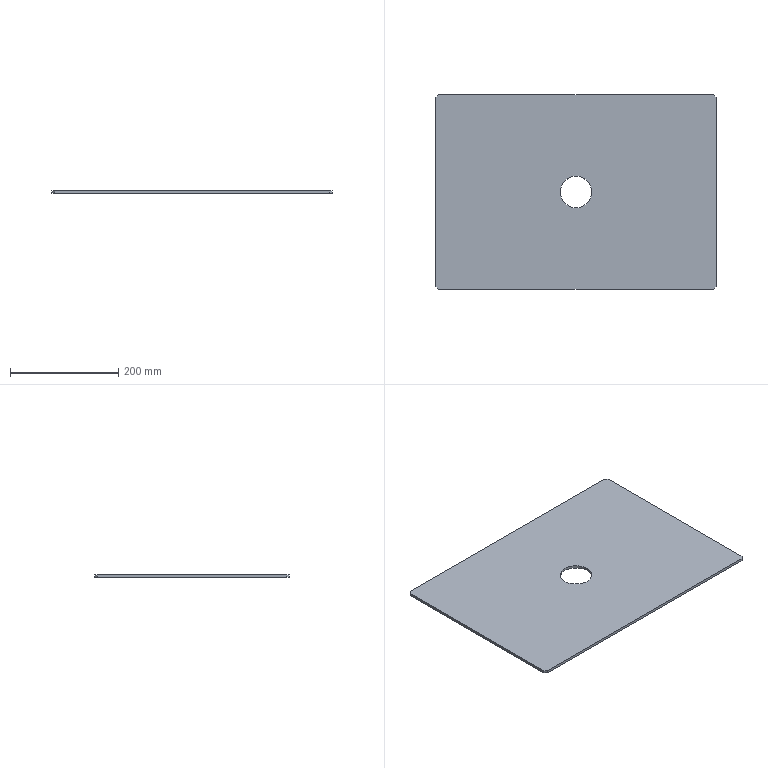Part | SolidWorks | features BaseBody 1 | 1 solid | 12 faces | box 518 x 360 x 5 mm | volume 918757 mm3 | plane 10 | cylinder 2 | commonest cylinder face diameters 58.4 x2
STEP:
#1=CARTESIAN_POINT('',(-29.2,0.,8.5));
#2=VERTEX_POINT('',#1);
#3=CARTESIAN_POINT('',(29.2,0.,8.5));
#4=VERTEX_POINT('',#3);
#5=CARTESIAN_POINT('',(0.,0.,8.5));
#6=DIRECTION('',(0.,0.,1.));
#7=DIRECTION('',(-1.,0.,0.));
#8=AXIS2_PLACEMENT_3D('',#5,#6,#7);
#9=CIRCLE('',#8,29.2);
#10=EDGE_CURVE('',#2,#4,#9,.T.);
#11=ORIENTED_EDGE('',*,*,#10,.T.);
#12=CARTESIAN_POINT('',(29.2,0.,3.5));
#13=VERTEX_POINT('',#12);
#14=CARTESIAN_POINT('',(29.2,0.,8.5));
#15=DIRECTION('',(0.,0.,-1.));
#16=VECTOR('',#15,1000.);
#17=LINE('',#14,#16);
#18=EDGE_CURVE('',#4,#13,#17,.T.);
#19=ORIENTED_EDGE('',*,*,#18,.T.);
#20=CARTESIAN_POINT('',(-29.2,0.,3.5));
#21=VERTEX_POINT('',#20);
#22=CARTESIAN_POINT('',(0.,0.,3.5));
#23=DIRECTION('',(0.,0.,1.));
#24=DIRECTION('',(-1.,0.,0.));
#25=AXIS2_PLACEMENT_3D('',#22,#23,#24);
#26=CIRCLE('',#25,29.2);
#27=EDGE_CURVE('',#21,#13,#26,.T.);
#28=ORIENTED_EDGE('',*,*,#27,.F.);
#29=CARTESIAN_POINT('',(-29.2,0.,8.5));
#30=DIRECTION('',(0.,0.,-1.));
#31=VECTOR('',#30,1000.);
#32=LINE('',#29,#31);
#33=EDGE_CURVE('',#2,#21,#32,.T.);
#34=ORIENTED_EDGE('',*,*,#33,.F.);
#35=EDGE_LOOP('',(#11,#19,#28,#34));
#36=FACE_OUTER_BOUND('',#35,.T.);
#37=CARTESIAN_POINT('',(0.,0.,8.5));
#38=DIRECTION('',(0.,0.,-1.));
#39=DIRECTION('',(-1.,0.,0.));
#40=AXIS2_PLACEMENT_3D('',#37,#38,#39);
#41=CYLINDRICAL_SURFACE('',#40,29.2);
#42=ADVANCED_FACE('',(#36),#41,.F.);
#43=ORIENTED_EDGE('',*,*,#10,.F.);
#44=CARTESIAN_POINT('',(0.,0.,8.5));
#45=DIRECTION('',(0.,0.,1.));
#46=DIRECTION('',(-1.,0.,0.));
#47=AXIS2_PLACEMENT_3D('',#44,#45,#46);
#48=CIRCLE('',#47,29.2);
#49=EDGE_CURVE('',#4,#2,#48,.T.);
#50=ORIENTED_EDGE('',*,*,#49,.F.);
#51=EDGE_LOOP('',(#43,#50));
#52=FACE_BOUND('',#51,.T.);
#53=CARTESIAN_POINT('',(-254.,180.,8.5));
#54=VERTEX_POINT('',#53);
#55=CARTESIAN_POINT('',(254.,180.,8.5));
#56=VERTEX_POINT('',#55);
#57=CARTESIAN_POINT('',(0.,180.,8.5));
#58=DIRECTION('',(1.,0.,0.));
#59=VECTOR('',#58,1000.);
#60=LINE('',#57,#59);
#61=EDGE_CURVE('',#54,#56,#60,.T.);
#62=ORIENTED_EDGE('',*,*,#61,.F.);
#63=CARTESIAN_POINT('',(-259.,175.,8.5));
#64=VERTEX_POINT('',#63);
#65=CARTESIAN_POINT('',(-259.,175.,8.5));
#66=DIRECTION('',(0.7071,0.7071,0.));
#67=VECTOR('',#66,1000.);
#68=LINE('',#65,#67);
#69=EDGE_CURVE('',#64,#54,#68,.T.);
#70=ORIENTED_EDGE('',*,*,#69,.F.);
#71=CARTESIAN_POINT('',(-259.,-175.,8.5));
#72=VERTEX_POINT('',#71);
#73=CARTESIAN_POINT('',(-259.,0.,8.5));
#74=DIRECTION('',(0.,1.,0.));
#75=VECTOR('',#74,1000.);
#76=LINE('',#73,#75);
#77=EDGE_CURVE('',#72,#64,#76,.T.);
#78=ORIENTED_EDGE('',*,*,#77,.F.);
#79=CARTESIAN_POINT('',(-254.,-180.,8.5));
#80=VERTEX_POINT('',#79);
#81=CARTESIAN_POINT('',(-254.,-180.,8.5));
#82=DIRECTION('',(-0.7071,0.7071,0.));
#83=VECTOR('',#82,1000.);
#84=LINE('',#81,#83);
#85=EDGE_CURVE('',#80,#72,#84,.T.);
#86=ORIENTED_EDGE('',*,*,#85,.F.);
#87=CARTESIAN_POINT('',(254.,-180.,8.5));
#88=VERTEX_POINT('',#87);
#89=CARTESIAN_POINT('',(0.,-180.,8.5));
#90=DIRECTION('',(-1.,0.,0.));
#91=VECTOR('',#90,1000.);
#92=LINE('',#89,#91);
#93=EDGE_CURVE('',#88,#80,#92,.T.);
#94=ORIENTED_EDGE('',*,*,#93,.F.);
#95=CARTESIAN_POINT('',(259.,-175.,8.5));
#96=VERTEX_POINT('',#95);
#97=CARTESIAN_POINT('',(259.,-175.,8.5));
#98=DIRECTION('',(-0.7071,-0.7071,0.));
#99=VECTOR('',#98,1000.);
#100=LINE('',#97,#99);
#101=EDGE_CURVE('',#96,#88,#100,.T.);
#102=ORIENTED_EDGE('',*,*,#101,.F.);
#103=CARTESIAN_POINT('',(259.,175.,8.5));
#104=VERTEX_POINT('',#103);
#105=CARTESIAN_POINT('',(259.,0.,8.5));
#106=DIRECTION('',(0.,-1.,0.));
#107=VECTOR('',#106,1000.);
#108=LINE('',#105,#107);
#109=EDGE_CURVE('',#104,#96,#108,.T.);
#110=ORIENTED_EDGE('',*,*,#109,.F.);
#111=CARTESIAN_POINT('',(254.,180.,8.5));
#112=DIRECTION('',(0.7071,-0.7071,0.));
#113=VECTOR('',#112,1000.);
#114=LINE('',#111,#113);
#115=EDGE_CURVE('',#56,#104,#114,.T.);
#116=ORIENTED_EDGE('',*,*,#115,.F.);
#117=EDGE_LOOP('',(#62,#70,#78,#86,#94,#102,#110,#116));
#118=FACE_OUTER_BOUND('',#117,.T.);
#119=CARTESIAN_POINT('',(0.,0.,8.5));
#120=DIRECTION('',(0.,0.,-1.));
#121=DIRECTION('',(-1.,0.,0.));
#122=AXIS2_PLACEMENT_3D('',#119,#120,#121);
#123=PLANE('',#122);
#124=ADVANCED_FACE('',(#52,#118),#123,.F.);
#125=ORIENTED_EDGE('',*,*,#18,.F.);
#126=ORIENTED_EDGE('',*,*,#49,.T.);
#127=ORIENTED_EDGE('',*,*,#33,.T.);
#128=CARTESIAN_POINT('',(0.,0.,3.5));
#129=DIRECTION('',(0.,0.,1.));
#130=DIRECTION('',(-1.,0.,0.));
#131=AXIS2_PLACEMENT_3D('',#128,#129,#130);
#132=CIRCLE('',#131,29.2);
#133=EDGE_CURVE('',#13,#21,#132,.T.);
#134=ORIENTED_EDGE('',*,*,#133,.F.);
#135=EDGE_LOOP('',(#125,#126,#127,#134));
#136=FACE_OUTER_BOUND('',#135,.T.);
#137=CARTESIAN_POINT('',(0.,0.,8.5));
#138=DIRECTION('',(0.,0.,-1.));
#139=DIRECTION('',(-1.,0.,0.));
#140=AXIS2_PLACEMENT_3D('',#137,#138,#139);
#141=CYLINDRICAL_SURFACE('',#140,29.2);
#142=ADVANCED_FACE('',(#136),#141,.F.);
#143=CARTESIAN_POINT('',(259.,175.,3.5));
#144=VERTEX_POINT('',#143);
#145=CARTESIAN_POINT('',(254.,180.,3.5));
#146=VERTEX_POINT('',#145);
#147=CARTESIAN_POINT('',(254.,180.,3.5));
#148=DIRECTION('',(-0.7071,0.7071,0.));
#149=VECTOR('',#148,1000.);
#150=LINE('',#147,#149);
#151=EDGE_CURVE('',#144,#146,#150,.T.);
#152=ORIENTED_EDGE('',*,*,#151,.T.);
#153=CARTESIAN_POINT('',(254.,180.,8.5));
#154=DIRECTION('',(0.,0.,1.));
#155=VECTOR('',#154,1000.);
#156=LINE('',#153,#155);
#157=EDGE_CURVE('',#146,#56,#156,.T.);
#158=ORIENTED_EDGE('',*,*,#157,.T.);
#159=ORIENTED_EDGE('',*,*,#115,.T.);
#160=CARTESIAN_POINT('',(259.,175.,8.5));
#161=DIRECTION('',(0.,0.,-1.));
#162=VECTOR('',#161,1000.);
#163=LINE('',#160,#162);
#164=EDGE_CURVE('',#104,#144,#163,.T.);
#165=ORIENTED_EDGE('',*,*,#164,.T.);
#166=EDGE_LOOP('',(#152,#158,#159,#165));
#167=FACE_OUTER_BOUND('',#166,.T.);
#168=CARTESIAN_POINT('',(254.,180.,8.5));
#169=DIRECTION('',(0.7071,0.7071,0.));
#170=DIRECTION('',(-0.7071,0.7071,0.));
#171=AXIS2_PLACEMENT_3D('',#168,#169,#170);
#172=PLANE('',#171);
#173=ADVANCED_FACE('',(#167),#172,.T.);
#174=CARTESIAN_POINT('',(-254.,180.,3.5));
#175=VERTEX_POINT('',#174);
#176=CARTESIAN_POINT('',(-254.,180.,3.5));
#177=DIRECTION('',(-1.,0.,0.));
#178=VECTOR('',#177,1000.);
#179=LINE('',#176,#178);
#180=EDGE_CURVE('',#146,#175,#179,.T.);
#181=ORIENTED_EDGE('',*,*,#180,.T.);
#182=CARTESIAN_POINT('',(-254.,180.,8.5));
#183=DIRECTION('',(0.,0.,1.));
#184=VECTOR('',#183,1000.);
#185=LINE('',#182,#184);
#186=EDGE_CURVE('',#175,#54,#185,.T.);
#187=ORIENTED_EDGE('',*,*,#186,.T.);
#188=ORIENTED_EDGE('',*,*,#61,.T.);
#189=ORIENTED_EDGE('',*,*,#157,.F.);
#190=EDGE_LOOP('',(#181,#187,#188,#189));
#191=FACE_OUTER_BOUND('',#190,.T.);
#192=CARTESIAN_POINT('',(-254.,180.,8.5));
#193=DIRECTION('',(0.,1.,0.));
#194=DIRECTION('',(0.,0.,1.));
#195=AXIS2_PLACEMENT_3D('',#192,#193,#194);
#196=PLANE('',#195);
#197=ADVANCED_FACE('',(#191),#196,.T.);
#198=CARTESIAN_POINT('',(-259.,175.,3.5));
#199=VERTEX_POINT('',#198);
#200=CARTESIAN_POINT('',(-259.,175.,3.5));
#201=DIRECTION('',(-0.7071,-0.7071,0.));
#202=VECTOR('',#201,1000.);
#203=LINE('',#200,#202);
#204=EDGE_CURVE('',#175,#199,#203,.T.);
#205=ORIENTED_EDGE('',*,*,#204,.T.);
#206=CARTESIAN_POINT('',(-259.,175.,8.5));
#207=DIRECTION('',(0.,0.,1.));
#208=VECTOR('',#207,1000.);
#209=LINE('',#206,#208);
#210=EDGE_CURVE('',#199,#64,#209,.T.);
#211=ORIENTED_EDGE('',*,*,#210,.T.);
#212=ORIENTED_EDGE('',*,*,#69,.T.);
#213=ORIENTED_EDGE('',*,*,#186,.F.);
#214=EDGE_LOOP('',(#205,#211,#212,#213));
#215=FACE_OUTER_BOUND('',#214,.T.);
#216=CARTESIAN_POINT('',(-259.,175.,8.5));
#217=DIRECTION('',(-0.7071,0.7071,0.));
#218=DIRECTION('',(-0.7071,-0.7071,0.));
#219=AXIS2_PLACEMENT_3D('',#216,#217,#218);
#220=PLANE('',#219);
#221=ADVANCED_FACE('',(#215),#220,.T.);
#222=CARTESIAN_POINT('',(-259.,-175.,3.5));
#223=VERTEX_POINT('',#222);
#224=CARTESIAN_POINT('',(-259.,-175.,3.5));
#225=DIRECTION('',(0.,-1.,0.));
#226=VECTOR('',#225,1000.);
#227=LINE('',#224,#226);
#228=EDGE_CURVE('',#199,#223,#227,.T.);
#229=ORIENTED_EDGE('',*,*,#228,.T.);
#230=CARTESIAN_POINT('',(-259.,-175.,8.5));
#231=DIRECTION('',(0.,0.,1.));
#232=VECTOR('',#231,1000.);
#233=LINE('',#230,#232);
#234=EDGE_CURVE('',#223,#72,#233,.T.);
#235=ORIENTED_EDGE('',*,*,#234,.T.);
#236=ORIENTED_EDGE('',*,*,#77,.T.);
#237=ORIENTED_EDGE('',*,*,#210,.F.);
#238=EDGE_LOOP('',(#229,#235,#236,#237));
#239=FACE_OUTER_BOUND('',#238,.T.);
#240=CARTESIAN_POINT('',(-259.,-175.,8.5));
#241=DIRECTION('',(-1.,0.,0.));
#242=DIRECTION('',(0.,0.,1.));
#243=AXIS2_PLACEMENT_3D('',#240,#241,#242);
#244=PLANE('',#243);
#245=ADVANCED_FACE('',(#239),#244,.T.);
#246=CARTESIAN_POINT('',(-254.,-180.,3.5));
#247=VERTEX_POINT('',#246);
#248=CARTESIAN_POINT('',(-254.,-180.,3.5));
#249=DIRECTION('',(0.7071,-0.7071,0.));
#250=VECTOR('',#249,1000.);
#251=LINE('',#248,#250);
#252=EDGE_CURVE('',#223,#247,#251,.T.);
#253=ORIENTED_EDGE('',*,*,#252,.T.);
#254=CARTESIAN_POINT('',(-254.,-180.,8.5));
#255=DIRECTION('',(0.,0.,1.));
#256=VECTOR('',#255,1000.);
#257=LINE('',#254,#256);
#258=EDGE_CURVE('',#247,#80,#257,.T.);
#259=ORIENTED_EDGE('',*,*,#258,.T.);
#260=ORIENTED_EDGE('',*,*,#85,.T.);
#261=ORIENTED_EDGE('',*,*,#234,.F.);
#262=EDGE_LOOP('',(#253,#259,#260,#261));
#263=FACE_OUTER_BOUND('',#262,.T.);
#264=CARTESIAN_POINT('',(-254.,-180.,8.5));
#265=DIRECTION('',(-0.7071,-0.7071,0.));
#266=DIRECTION('',(0.7071,-0.7071,0.));
#267=AXIS2_PLACEMENT_3D('',#264,#265,#266);
#268=PLANE('',#267);
#269=ADVANCED_FACE('',(#263),#268,.T.);
#270=CARTESIAN_POINT('',(254.,-180.,3.5));
#271=VERTEX_POINT('',#270);
#272=CARTESIAN_POINT('',(254.,-180.,3.5));
#273=DIRECTION('',(1.,0.,0.));
#274=VECTOR('',#273,1000.);
#275=LINE('',#272,#274);
#276=EDGE_CURVE('',#247,#271,#275,.T.);
#277=ORIENTED_EDGE('',*,*,#276,.T.);
#278=CARTESIAN_POINT('',(254.,-180.,8.5));
#279=DIRECTION('',(0.,0.,1.));
#280=VECTOR('',#279,1000.);
#281=LINE('',#278,#280);
#282=EDGE_CURVE('',#271,#88,#281,.T.);
#283=ORIENTED_EDGE('',*,*,#282,.T.);
#284=ORIENTED_EDGE('',*,*,#93,.T.);
#285=ORIENTED_EDGE('',*,*,#258,.F.);
#286=EDGE_LOOP('',(#277,#283,#284,#285));
#287=FACE_OUTER_BOUND('',#286,.T.);
#288=CARTESIAN_POINT('',(254.,-180.,8.5));
#289=DIRECTION('',(0.,-1.,0.));
#290=DIRECTION('',(1.,0.,0.));
#291=AXIS2_PLACEMENT_3D('',#288,#289,#290);
#292=PLANE('',#291);
#293=ADVANCED_FACE('',(#287),#292,.T.);
#294=CARTESIAN_POINT('',(259.,-175.,3.5));
#295=VERTEX_POINT('',#294);
#296=CARTESIAN_POINT('',(259.,-175.,3.5));
#297=DIRECTION('',(0.7071,0.7071,0.));
#298=VECTOR('',#297,1000.);
#299=LINE('',#296,#298);
#300=EDGE_CURVE('',#271,#295,#299,.T.);
#301=ORIENTED_EDGE('',*,*,#300,.T.);
#302=CARTESIAN_POINT('',(259.,-175.,8.5));
#303=DIRECTION('',(0.,0.,1.));
#304=VECTOR('',#303,1000.);
#305=LINE('',#302,#304);
#306=EDGE_CURVE('',#295,#96,#305,.T.);
#307=ORIENTED_EDGE('',*,*,#306,.T.);
#308=ORIENTED_EDGE('',*,*,#101,.T.);
#309=ORIENTED_EDGE('',*,*,#282,.F.);
#310=EDGE_LOOP('',(#301,#307,#308,#309));
#311=FACE_OUTER_BOUND('',#310,.T.);
#312=CARTESIAN_POINT('',(259.,-175.,8.5));
#313=DIRECTION('',(0.7071,-0.7071,0.));
#314=DIRECTION('',(0.7071,0.7071,0.));
#315=AXIS2_PLACEMENT_3D('',#312,#313,#314);
#316=PLANE('',#315);
#317=ADVANCED_FACE('',(#311),#316,.T.);
#318=CARTESIAN_POINT('',(259.,175.,3.5));
#319=DIRECTION('',(0.,1.,0.));
#320=VECTOR('',#319,1000.);
#321=LINE('',#318,#320);
#322=EDGE_CURVE('',#295,#144,#321,.T.);
#323=ORIENTED_EDGE('',*,*,#322,.T.);
#324=ORIENTED_EDGE('',*,*,#164,.F.);
#325=ORIENTED_EDGE('',*,*,#109,.T.);
#326=ORIENTED_EDGE('',*,*,#306,.F.);
#327=EDGE_LOOP('',(#323,#324,#325,#326));
#328=FACE_OUTER_BOUND('',#327,.T.);
#329=CARTESIAN_POINT('',(259.,175.,8.5));
#330=DIRECTION('',(1.,0.,0.));
#331=DIRECTION('',(0.,0.,-1.));
#332=AXIS2_PLACEMENT_3D('',#329,#330,#331);
#333=PLANE('',#332);
#334=ADVANCED_FACE('',(#328),#333,.T.);
#335=ORIENTED_EDGE('',*,*,#27,.T.);
#336=ORIENTED_EDGE('',*,*,#133,.T.);
#337=EDGE_LOOP('',(#335,#336));
#338=FACE_BOUND('',#337,.T.);
#339=ORIENTED_EDGE('',*,*,#204,.F.);
#340=ORIENTED_EDGE('',*,*,#180,.F.);
#341=ORIENTED_EDGE('',*,*,#151,.F.);
#342=ORIENTED_EDGE('',*,*,#322,.F.);
#343=ORIENTED_EDGE('',*,*,#300,.F.);
#344=ORIENTED_EDGE('',*,*,#276,.F.);
#345=ORIENTED_EDGE('',*,*,#252,.F.);
#346=ORIENTED_EDGE('',*,*,#228,.F.);
#347=EDGE_LOOP('',(#339,#340,#341,#342,#343,#344,#345,#346));
#348=FACE_OUTER_BOUND('',#347,.T.);
#349=CARTESIAN_POINT('',(0.,0.,3.5));
#350=DIRECTION('',(0.,0.,-1.));
#351=DIRECTION('',(-1.,0.,0.));
#352=AXIS2_PLACEMENT_3D('',#349,#350,#351);
#353=PLANE('',#352);
#354=ADVANCED_FACE('',(#338,#348),#353,.T.);
#355=CLOSED_SHELL('',(#42,#124,#142,#173,#197,#221,#245,#269,#293,#317,#334,#354));
#356=MANIFOLD_SOLID_BREP('',#355);
#357=CARTESIAN_POINT('',(0.,0.,0.));
#358=DIRECTION('',(0.,0.,1.));
#359=DIRECTION('',(1.,0.,0.));
#360=AXIS2_PLACEMENT_3D('',#357,#358,#359);
#361=(LENGTH_UNIT()NAMED_UNIT(*)SI_UNIT(.MILLI.,.METRE.));
#362=UNCERTAINTY_MEASURE_WITH_UNIT(LENGTH_MEASURE(0.00001),#361,'','');
#363=(NAMED_UNIT(*)PLANE_ANGLE_UNIT()SI_UNIT($,.RADIAN.));
#364=(NAMED_UNIT(*)SI_UNIT($,.STERADIAN.)SOLID_ANGLE_UNIT());
#365=(GEOMETRIC_REPRESENTATION_CONTEXT(3)GLOBAL_UNCERTAINTY_ASSIGNED_CONTEXT((#362))GLOBAL_UNIT_ASSIGNED_CONTEXT((#361,#363,#364))REPRESENTATION_CONTEXT('',''));
#366=ADVANCED_BREP_SHAPE_REPRESENTATION('',(#356,#360),#365);